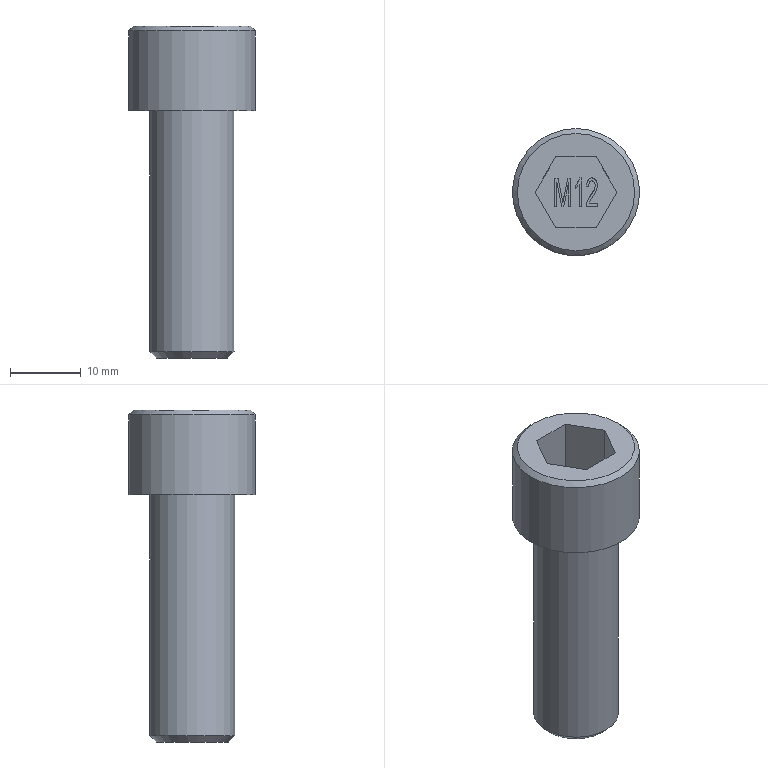Part | STEP file | M12-1 | 1 solid | 43 faces | box 18 x 18 x 47 mm | volume 6292 mm3 | plane 33 | other 6 | cone 2 | cylinder 2 | commonest cylinder face diameters 12 x1 18 x1